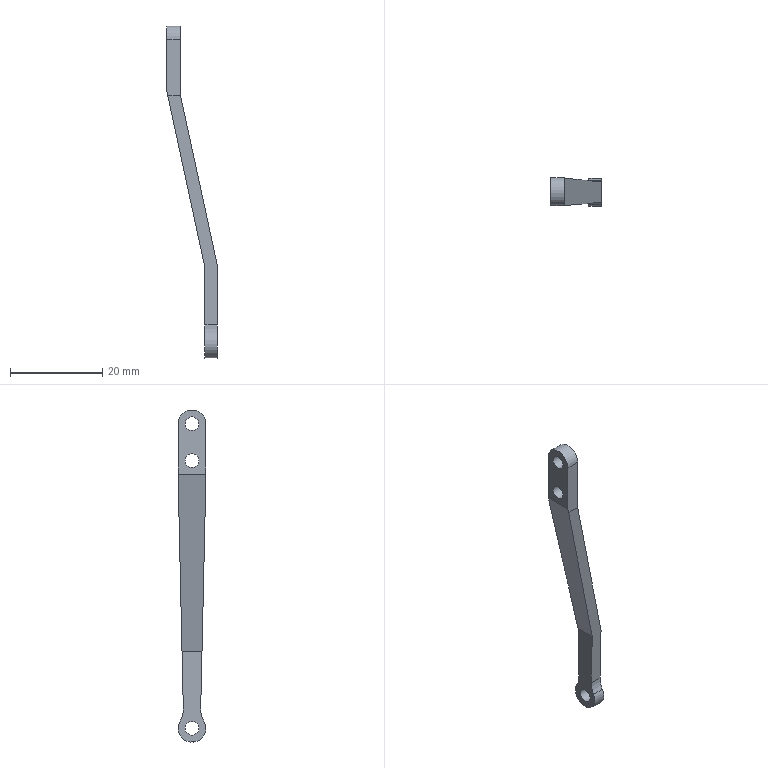Part | STEP file | 2-18 | 1 solid | 17 faces | box 11 x 6 x 72 mm | volume 957.208 mm3 | plane 10 | cylinder 7 | commonest cylinder face diameters 3 x3 6 x2 10 x2
STEP:
#1=CARTESIAN_POINT('',(0.,0.,0.));
#2=DIRECTION('',(0.,0.,1.));
#3=DIRECTION('',(1.,0.,0.));
#4=AXIS2_PLACEMENT_3D('',#1,#2,#3);
#5=CARTESIAN_POINT('',(-7.5,3.,0.));
#6=VERTEX_POINT('',#5);
#7=CARTESIAN_POINT('',(-7.5,-3.,0.));
#8=VERTEX_POINT('',#7);
#9=CARTESIAN_POINT('',(-7.5,0.,0.));
#10=DIRECTION('',(1.,0.,0.));
#11=DIRECTION('',(0.,1.,0.));
#12=AXIS2_PLACEMENT_3D('',#9,#10,#11);
#13=CIRCLE('',#12,3.);
#14=CARTESIAN_POINT('',(-7.5,32.591,-33.464));
#15=DIRECTION('',(1.,0.,0.));
#16=DIRECTION('',(0.,1.,0.));
#17=AXIS2_PLACEMENT_3D('',#14,#15,#16);
#18=PLANE('',#17);
#19=CARTESIAN_POINT('',(-32.591,33.464));
#20=DIRECTION('',(1.,0.));
#21=AXIS2_PLACEMENT_2D('',#19,#20);
#22=CIRCLE('',#21,3.);
#23=(GEOMETRIC_REPRESENTATION_CONTEXT(2)PARAMETRIC_REPRESENTATION_CONTEXT()REPRESENTATION_CONTEXT('',''));
#24=DEFINITIONAL_REPRESENTATION('',(#22),#23);
#25=PCURVE('',#18,#24);
#26=CARTESIAN_POINT('',(7.5,0.,0.));
#27=DIRECTION('',(-1.,0.,0.));
#28=DIRECTION('',(0.,1.,0.));
#29=AXIS2_PLACEMENT_3D('',#26,#27,#28);
#30=CYLINDRICAL_SURFACE('',#29,3.);
#31=CARTESIAN_POINT('',(6.283,15.));
#32=DIRECTION('',(-1.,0.));
#33=VECTOR('',#32,1.);
#34=LINE('',#31,#33);
#35=(GEOMETRIC_REPRESENTATION_CONTEXT(2)PARAMETRIC_REPRESENTATION_CONTEXT()REPRESENTATION_CONTEXT('',''));
#36=DEFINITIONAL_REPRESENTATION('',(#34),#35);
#37=PCURVE('',#30,#36);
#38=SURFACE_CURVE('',#13,(#25,#37),.PCURVE_S1.);
#39=EDGE_CURVE('',#6,#8,#38,.T.);
#40=ORIENTED_EDGE('',*,*,#39,.T.);
#41=CARTESIAN_POINT('',(-7.5,-3.,-10.901));
#42=VERTEX_POINT('',#41);
#43=CARTESIAN_POINT('',(-7.5,-3.,0.));
#44=DIRECTION('',(0.,0.,-1.));
#45=VECTOR('',#44,1.);
#46=LINE('',#43,#45);
#47=CARTESIAN_POINT('',(-35.591,33.464));
#48=DIRECTION('',(0.,-1.));
#49=VECTOR('',#48,1.);
#50=LINE('',#47,#49);
#51=(GEOMETRIC_REPRESENTATION_CONTEXT(2)PARAMETRIC_REPRESENTATION_CONTEXT()REPRESENTATION_CONTEXT('',''));
#52=DEFINITIONAL_REPRESENTATION('',(#50),#51);
#53=PCURVE('',#18,#52);
#54=CARTESIAN_POINT('',(0.,-3.,-6.));
#55=DIRECTION('',(0.,1.,0.));
#56=DIRECTION('',(0.,0.,-1.));
#57=AXIS2_PLACEMENT_3D('',#54,#55,#56);
#58=PLANE('',#57);
#59=CARTESIAN_POINT('',(-6.,7.5));
#60=DIRECTION('',(1.,0.));
#61=VECTOR('',#60,1.);
#62=LINE('',#59,#61);
#63=(GEOMETRIC_REPRESENTATION_CONTEXT(2)PARAMETRIC_REPRESENTATION_CONTEXT()REPRESENTATION_CONTEXT('',''));
#64=DEFINITIONAL_REPRESENTATION('',(#62),#63);
#65=PCURVE('',#58,#64);
#66=SURFACE_CURVE('',#46,(#53,#65),.PCURVE_S1.);
#67=EDGE_CURVE('',#8,#42,#66,.T.);
#68=ORIENTED_EDGE('',*,*,#67,.T.);
#69=CARTESIAN_POINT('',(-7.5,3.,-10.901));
#70=VERTEX_POINT('',#69);
#71=CARTESIAN_POINT('',(-7.5,3.,-10.901));
#72=DIRECTION('',(0.,-1.,0.));
#73=VECTOR('',#72,1.);
#74=LINE('',#71,#73);
#75=CARTESIAN_POINT('',(-29.591,22.563));
#76=DIRECTION('',(-1.,0.));
#77=VECTOR('',#76,1.);
#78=LINE('',#75,#77);
#79=(GEOMETRIC_REPRESENTATION_CONTEXT(2)PARAMETRIC_REPRESENTATION_CONTEXT()REPRESENTATION_CONTEXT('',''));
#80=DEFINITIONAL_REPRESENTATION('',(#78),#79);
#81=PCURVE('',#18,#80);
#82=CARTESIAN_POINT('',(-3.35,0.,-30.095));
#83=DIRECTION('',(-0.9774,0.,-0.2113));
#84=DIRECTION('',(0.2113,0.,-0.9774));
#85=AXIS2_PLACEMENT_3D('',#82,#83,#84);
#86=PLANE('',#85);
#87=CARTESIAN_POINT('',(-19.637,-3.));
#88=DIRECTION('',(0.,1.));
#89=VECTOR('',#88,1.);
#90=LINE('',#87,#89);
#91=(GEOMETRIC_REPRESENTATION_CONTEXT(2)PARAMETRIC_REPRESENTATION_CONTEXT()REPRESENTATION_CONTEXT('',''));
#92=DEFINITIONAL_REPRESENTATION('',(#90),#91);
#93=PCURVE('',#86,#92);
#94=SURFACE_CURVE('',#74,(#81,#93),.PCURVE_S1.);
#95=EDGE_CURVE('',#70,#42,#94,.T.);
#96=ORIENTED_EDGE('',*,*,#95,.F.);
#97=CARTESIAN_POINT('',(-7.5,3.,-10.901));
#98=DIRECTION('',(0.,0.,1.));
#99=VECTOR('',#98,1.);
#100=LINE('',#97,#99);
#101=CARTESIAN_POINT('',(-29.591,22.563));
#102=DIRECTION('',(0.,1.));
#103=VECTOR('',#102,1.);
#104=LINE('',#101,#103);
#105=(GEOMETRIC_REPRESENTATION_CONTEXT(2)PARAMETRIC_REPRESENTATION_CONTEXT()REPRESENTATION_CONTEXT('',''));
#106=DEFINITIONAL_REPRESENTATION('',(#104),#105);
#107=PCURVE('',#18,#106);
#108=CARTESIAN_POINT('',(0.,3.,-6.));
#109=DIRECTION('',(0.,-1.,0.));
#110=DIRECTION('',(0.,0.,1.));
#111=AXIS2_PLACEMENT_3D('',#108,#109,#110);
#112=PLANE('',#111);
#113=CARTESIAN_POINT('',(-4.901,7.5));
#114=DIRECTION('',(1.,0.));
#115=VECTOR('',#114,1.);
#116=LINE('',#113,#115);
#117=(GEOMETRIC_REPRESENTATION_CONTEXT(2)PARAMETRIC_REPRESENTATION_CONTEXT()REPRESENTATION_CONTEXT('',''));
#118=DEFINITIONAL_REPRESENTATION('',(#116),#117);
#119=PCURVE('',#112,#118);
#120=SURFACE_CURVE('',#100,(#107,#119),.PCURVE_S1.);
#121=EDGE_CURVE('',#70,#6,#120,.T.);
#122=ORIENTED_EDGE('',*,*,#121,.T.);
#123=EDGE_LOOP('',(#40,#68,#96,#122));
#124=FACE_BOUND('',#123,.F.);
#125=CARTESIAN_POINT('',(-7.5,1.5,0.));
#126=VERTEX_POINT('',#125);
#127=CARTESIAN_POINT('',(-7.5,0.,0.));
#128=DIRECTION('',(-1.,0.,0.));
#129=DIRECTION('',(0.,1.,0.));
#130=AXIS2_PLACEMENT_3D('',#127,#128,#129);
#131=CIRCLE('',#130,1.5);
#132=CARTESIAN_POINT('',(-31.091,33.464));
#133=CARTESIAN_POINT('',(-31.091,30.866));
#134=CARTESIAN_POINT('',(-33.341,32.165));
#135=CARTESIAN_POINT('',(-35.591,33.464));
#136=CARTESIAN_POINT('',(-33.341,34.763));
#137=CARTESIAN_POINT('',(-31.091,36.062));
#138=CARTESIAN_POINT('',(-31.091,33.464));
#139=(BOUNDED_CURVE()B_SPLINE_CURVE(2,(#132,#133,#134,#135,#136,#137,#138),.UNSPECIFIED.,.T.,.F.)B_SPLINE_CURVE_WITH_KNOTS((1,2,2,2,2,1),(-2.094,0.,2.094,4.189,6.283,8.378),.UNSPECIFIED.)CURVE()GEOMETRIC_REPRESENTATION_ITEM()RATIONAL_B_SPLINE_CURVE((1.,0.5,1.,0.5,1.,0.5,1.))REPRESENTATION_ITEM(''));
#140=(GEOMETRIC_REPRESENTATION_CONTEXT(2)PARAMETRIC_REPRESENTATION_CONTEXT()REPRESENTATION_CONTEXT('',''));
#141=DEFINITIONAL_REPRESENTATION('',(#139),#140);
#142=PCURVE('',#18,#141);
#143=CARTESIAN_POINT('',(7.5,0.,0.));
#144=DIRECTION('',(-1.,0.,0.));
#145=DIRECTION('',(0.,1.,0.));
#146=AXIS2_PLACEMENT_3D('',#143,#144,#145);
#147=CYLINDRICAL_SURFACE('',#146,1.5);
#148=CARTESIAN_POINT('',(0.,15.));
#149=DIRECTION('',(1.,0.));
#150=VECTOR('',#149,1.);
#151=LINE('',#148,#150);
#152=(GEOMETRIC_REPRESENTATION_CONTEXT(2)PARAMETRIC_REPRESENTATION_CONTEXT()REPRESENTATION_CONTEXT('',''));
#153=DEFINITIONAL_REPRESENTATION('',(#151),#152);
#154=PCURVE('',#147,#153);
#155=SURFACE_CURVE('',#131,(#142,#154),.PCURVE_S1.);
#156=EDGE_CURVE('',#126,#126,#155,.T.);
#157=ORIENTED_EDGE('',*,*,#156,.T.);
#158=EDGE_LOOP('',(#157));
#159=FACE_BOUND('',#158,.F.);
#160=CARTESIAN_POINT('',(-7.5,1.5,-8.));
#161=VERTEX_POINT('',#160);
#162=CARTESIAN_POINT('',(-7.5,0.,-8.));
#163=DIRECTION('',(-1.,0.,0.));
#164=DIRECTION('',(0.,1.,0.));
#165=AXIS2_PLACEMENT_3D('',#162,#163,#164);
#166=CIRCLE('',#165,1.5);
#167=CARTESIAN_POINT('',(-31.091,25.464));
#168=CARTESIAN_POINT('',(-31.091,22.866));
#169=CARTESIAN_POINT('',(-33.341,24.165));
#170=CARTESIAN_POINT('',(-35.591,25.464));
#171=CARTESIAN_POINT('',(-33.341,26.763));
#172=CARTESIAN_POINT('',(-31.091,28.062));
#173=CARTESIAN_POINT('',(-31.091,25.464));
#174=(BOUNDED_CURVE()B_SPLINE_CURVE(2,(#167,#168,#169,#170,#171,#172,#173),.UNSPECIFIED.,.T.,.F.)B_SPLINE_CURVE_WITH_KNOTS((1,2,2,2,2,1),(-2.094,0.,2.094,4.189,6.283,8.378),.UNSPECIFIED.)CURVE()GEOMETRIC_REPRESENTATION_ITEM()RATIONAL_B_SPLINE_CURVE((1.,0.5,1.,0.5,1.,0.5,1.))REPRESENTATION_ITEM(''));
#175=(GEOMETRIC_REPRESENTATION_CONTEXT(2)PARAMETRIC_REPRESENTATION_CONTEXT()REPRESENTATION_CONTEXT('',''));
#176=DEFINITIONAL_REPRESENTATION('',(#174),#175);
#177=PCURVE('',#18,#176);
#178=CARTESIAN_POINT('',(7.5,0.,-8.));
#179=DIRECTION('',(-1.,0.,0.));
#180=DIRECTION('',(0.,1.,0.));
#181=AXIS2_PLACEMENT_3D('',#178,#179,#180);
#182=CYLINDRICAL_SURFACE('',#181,1.5);
#183=CARTESIAN_POINT('',(0.,15.));
#184=DIRECTION('',(1.,0.));
#185=VECTOR('',#184,1.);
#186=LINE('',#183,#185);
#187=(GEOMETRIC_REPRESENTATION_CONTEXT(2)PARAMETRIC_REPRESENTATION_CONTEXT()REPRESENTATION_CONTEXT('',''));
#188=DEFINITIONAL_REPRESENTATION('',(#186),#187);
#189=PCURVE('',#182,#188);
#190=SURFACE_CURVE('',#166,(#177,#189),.PCURVE_S1.);
#191=EDGE_CURVE('',#161,#161,#190,.T.);
#192=ORIENTED_EDGE('',*,*,#191,.T.);
#193=EDGE_LOOP('',(#192));
#194=FACE_BOUND('',#193,.F.);
#195=ADVANCED_FACE('',(#124,#159,#194),#18,.F.);
#196=CARTESIAN_POINT('',(-4.5,-3.,0.));
#197=VERTEX_POINT('',#196);
#198=CARTESIAN_POINT('',(-4.5,-3.,0.));
#199=DIRECTION('',(-1.,0.,0.));
#200=VECTOR('',#199,1.);
#201=LINE('',#198,#200);
#202=CARTESIAN_POINT('',(3.142,12.));
#203=DIRECTION('',(0.,1.));
#204=VECTOR('',#203,1.);
#205=LINE('',#202,#204);
#206=(GEOMETRIC_REPRESENTATION_CONTEXT(2)PARAMETRIC_REPRESENTATION_CONTEXT()REPRESENTATION_CONTEXT('',''));
#207=DEFINITIONAL_REPRESENTATION('',(#205),#206);
#208=PCURVE('',#30,#207);
#209=CARTESIAN_POINT('',(-6.,4.5));
#210=DIRECTION('',(0.,1.));
#211=VECTOR('',#210,1.);
#212=LINE('',#209,#211);
#213=(GEOMETRIC_REPRESENTATION_CONTEXT(2)PARAMETRIC_REPRESENTATION_CONTEXT()REPRESENTATION_CONTEXT('',''));
#214=DEFINITIONAL_REPRESENTATION('',(#212),#213);
#215=PCURVE('',#58,#214);
#216=SURFACE_CURVE('',#201,(#208,#215),.PCURVE_S1.);
#217=EDGE_CURVE('',#197,#8,#216,.T.);
#218=ORIENTED_EDGE('',*,*,#217,.F.);
#219=CARTESIAN_POINT('',(-4.5,3.,0.));
#220=VERTEX_POINT('',#219);
#221=CARTESIAN_POINT('',(-4.5,0.,0.));
#222=DIRECTION('',(1.,0.,0.));
#223=DIRECTION('',(0.,1.,0.));
#224=AXIS2_PLACEMENT_3D('',#221,#222,#223);
#225=CIRCLE('',#224,3.);
#226=CARTESIAN_POINT('',(6.283,12.));
#227=DIRECTION('',(-1.,0.));
#228=VECTOR('',#227,1.);
#229=LINE('',#226,#228);
#230=(GEOMETRIC_REPRESENTATION_CONTEXT(2)PARAMETRIC_REPRESENTATION_CONTEXT()REPRESENTATION_CONTEXT('',''));
#231=DEFINITIONAL_REPRESENTATION('',(#229),#230);
#232=PCURVE('',#30,#231);
#233=CARTESIAN_POINT('',(-4.5,0.,-4.5));
#234=DIRECTION('',(1.,0.,0.));
#235=DIRECTION('',(0.,0.,1.));
#236=AXIS2_PLACEMENT_3D('',#233,#234,#235);
#237=PLANE('',#236);
#238=CARTESIAN_POINT('',(4.5,0.));
#239=DIRECTION('',(0.,-1.));
#240=AXIS2_PLACEMENT_2D('',#238,#239);
#241=CIRCLE('',#240,3.);
#242=(GEOMETRIC_REPRESENTATION_CONTEXT(2)PARAMETRIC_REPRESENTATION_CONTEXT()REPRESENTATION_CONTEXT('',''));
#243=DEFINITIONAL_REPRESENTATION('',(#241),#242);
#244=PCURVE('',#237,#243);
#245=SURFACE_CURVE('',#225,(#232,#244),.PCURVE_S1.);
#246=EDGE_CURVE('',#220,#197,#245,.T.);
#247=ORIENTED_EDGE('',*,*,#246,.F.);
#248=CARTESIAN_POINT('',(-4.5,3.,0.));
#249=DIRECTION('',(-1.,0.,0.));
#250=VECTOR('',#249,1.);
#251=LINE('',#248,#250);
#252=CARTESIAN_POINT('',(6.283,12.));
#253=DIRECTION('',(0.,1.));
#254=VECTOR('',#253,1.);
#255=LINE('',#252,#254);
#256=(GEOMETRIC_REPRESENTATION_CONTEXT(2)PARAMETRIC_REPRESENTATION_CONTEXT()REPRESENTATION_CONTEXT('',''));
#257=DEFINITIONAL_REPRESENTATION('',(#255),#256);
#258=PCURVE('',#30,#257);
#259=CARTESIAN_POINT('',(6.,4.5));
#260=DIRECTION('',(0.,1.));
#261=VECTOR('',#260,1.);
#262=LINE('',#259,#261);
#263=(GEOMETRIC_REPRESENTATION_CONTEXT(2)PARAMETRIC_REPRESENTATION_CONTEXT()REPRESENTATION_CONTEXT('',''));
#264=DEFINITIONAL_REPRESENTATION('',(#262),#263);
#265=PCURVE('',#112,#264);
#266=SURFACE_CURVE('',#251,(#258,#265),.PCURVE_S1.);
#267=EDGE_CURVE('',#220,#6,#266,.T.);
#268=ORIENTED_EDGE('',*,*,#267,.T.);
#269=ORIENTED_EDGE('',*,*,#39,.T.);
#270=EDGE_LOOP('',(#218,#247,#268,#269));
#271=FACE_BOUND('',#270,.T.);
#272=ADVANCED_FACE('',(#271),#30,.T.);
#273=ORIENTED_EDGE('',*,*,#217,.F.);
#274=CARTESIAN_POINT('',(-4.5,-3.,-12.));
#275=VERTEX_POINT('',#274);
#276=CARTESIAN_POINT('',(-4.5,-3.,0.));
#277=DIRECTION('',(0.,0.,-1.));
#278=VECTOR('',#277,1.);
#279=LINE('',#276,#278);
#280=CARTESIAN_POINT('',(-6.,4.5));
#281=DIRECTION('',(1.,0.));
#282=VECTOR('',#281,1.);
#283=LINE('',#280,#282);
#284=(GEOMETRIC_REPRESENTATION_CONTEXT(2)PARAMETRIC_REPRESENTATION_CONTEXT()REPRESENTATION_CONTEXT('',''));
#285=DEFINITIONAL_REPRESENTATION('',(#283),#284);
#286=PCURVE('',#58,#285);
#287=CARTESIAN_POINT('',(4.5,3.));
#288=DIRECTION('',(-1.,0.));
#289=VECTOR('',#288,1.);
#290=LINE('',#287,#289);
#291=(GEOMETRIC_REPRESENTATION_CONTEXT(2)PARAMETRIC_REPRESENTATION_CONTEXT()REPRESENTATION_CONTEXT('',''));
#292=DEFINITIONAL_REPRESENTATION('',(#290),#291);
#293=PCURVE('',#237,#292);
#294=SURFACE_CURVE('',#279,(#286,#293),.PCURVE_S1.);
#295=EDGE_CURVE('',#197,#275,#294,.T.);
#296=ORIENTED_EDGE('',*,*,#295,.T.);
#297=CARTESIAN_POINT('',(-7.262,-3.,-12.));
#298=VERTEX_POINT('',#297);
#299=CARTESIAN_POINT('',(-4.5,-3.,-12.));
#300=DIRECTION('',(-1.,0.,0.));
#301=VECTOR('',#300,1.);
#302=LINE('',#299,#301);
#303=CARTESIAN_POINT('',(6.,4.5));
#304=DIRECTION('',(0.,1.));
#305=VECTOR('',#304,1.);
#306=LINE('',#303,#305);
#307=(GEOMETRIC_REPRESENTATION_CONTEXT(2)PARAMETRIC_REPRESENTATION_CONTEXT()REPRESENTATION_CONTEXT('',''));
#308=DEFINITIONAL_REPRESENTATION('',(#306),#307);
#309=PCURVE('',#58,#308);
#310=CARTESIAN_POINT('',(0.,-2.443,-36.907));
#311=DIRECTION('',(0.,0.9997,0.02236));
#312=DIRECTION('',(0.,0.02236,-0.9997));
#313=AXIS2_PLACEMENT_3D('',#310,#311,#312);
#314=PLANE('',#313);
#315=CARTESIAN_POINT('',(-24.913,4.5));
#316=DIRECTION('',(0.,1.));
#317=VECTOR('',#316,1.);
#318=LINE('',#315,#317);
#319=(GEOMETRIC_REPRESENTATION_CONTEXT(2)PARAMETRIC_REPRESENTATION_CONTEXT()REPRESENTATION_CONTEXT('',''));
#320=DEFINITIONAL_REPRESENTATION('',(#318),#319);
#321=PCURVE('',#314,#320);
#322=SURFACE_CURVE('',#302,(#309,#321),.PCURVE_S1.);
#323=EDGE_CURVE('',#275,#298,#322,.T.);
#324=ORIENTED_EDGE('',*,*,#323,.T.);
#325=CARTESIAN_POINT('',(-7.262,-3.,-12.));
#326=DIRECTION('',(-0.2113,0.,0.9774));
#327=VECTOR('',#326,1.);
#328=LINE('',#325,#327);
#329=CARTESIAN_POINT('',(6.,7.262));
#330=DIRECTION('',(-0.9774,0.2113));
#331=VECTOR('',#330,1.);
#332=LINE('',#329,#331);
#333=(GEOMETRIC_REPRESENTATION_CONTEXT(2)PARAMETRIC_REPRESENTATION_CONTEXT()REPRESENTATION_CONTEXT('',''));
#334=DEFINITIONAL_REPRESENTATION('',(#332),#333);
#335=PCURVE('',#58,#334);
#336=CARTESIAN_POINT('',(-18.513,3.));
#337=DIRECTION('',(-1.,0.));
#338=VECTOR('',#337,1.);
#339=LINE('',#336,#338);
#340=(GEOMETRIC_REPRESENTATION_CONTEXT(2)PARAMETRIC_REPRESENTATION_CONTEXT()REPRESENTATION_CONTEXT('',''));
#341=DEFINITIONAL_REPRESENTATION('',(#339),#340);
#342=PCURVE('',#86,#341);
#343=SURFACE_CURVE('',#328,(#335,#342),.PCURVE_S1.);
#344=EDGE_CURVE('',#298,#42,#343,.T.);
#345=ORIENTED_EDGE('',*,*,#344,.T.);
#346=ORIENTED_EDGE('',*,*,#67,.F.);
#347=EDGE_LOOP('',(#273,#296,#324,#345,#346));
#348=FACE_BOUND('',#347,.F.);
#349=ADVANCED_FACE('',(#348),#58,.F.);
#350=ORIENTED_EDGE('',*,*,#323,.F.);
#351=CARTESIAN_POINT('',(3.5,-2.172,-49.));
#352=VERTEX_POINT('',#351);
#353=CARTESIAN_POINT('',(-4.5,-3.,-12.));
#354=DIRECTION('',(0.2113,0.02186,-0.9772));
#355=VECTOR('',#354,1.);
#356=LINE('',#353,#355);
#357=CARTESIAN_POINT('',(-24.913,4.5));
#358=DIRECTION('',(0.9774,-0.2113));
#359=VECTOR('',#358,1.);
#360=LINE('',#357,#359);
#361=(GEOMETRIC_REPRESENTATION_CONTEXT(2)PARAMETRIC_REPRESENTATION_CONTEXT()REPRESENTATION_CONTEXT('',''));
#362=DEFINITIONAL_REPRESENTATION('',(#360),#361);
#363=PCURVE('',#314,#362);
#364=CARTESIAN_POINT('',(-0.5,0.,-30.5));
#365=DIRECTION('',(0.9774,0.,0.2113));
#366=DIRECTION('',(-0.2113,0.,0.9774));
#367=AXIS2_PLACEMENT_3D('',#364,#365,#366);
#368=PLANE('',#367);
#369=CARTESIAN_POINT('',(18.927,3.));
#370=DIRECTION('',(-0.9998,-0.02186));
#371=VECTOR('',#370,1.);
#372=LINE('',#369,#371);
#373=(GEOMETRIC_REPRESENTATION_CONTEXT(2)PARAMETRIC_REPRESENTATION_CONTEXT()REPRESENTATION_CONTEXT('',''));
#374=DEFINITIONAL_REPRESENTATION('',(#372),#373);
#375=PCURVE('',#368,#374);
#376=SURFACE_CURVE('',#356,(#363,#375),.PCURVE_S1.);
#377=EDGE_CURVE('',#275,#352,#376,.T.);
#378=ORIENTED_EDGE('',*,*,#377,.T.);
#379=CARTESIAN_POINT('',(3.5,-1.886,-61.814));
#380=VERTEX_POINT('',#379);
#381=CARTESIAN_POINT('',(3.5,-2.172,-49.));
#382=DIRECTION('',(0.,0.02236,-0.9997));
#383=VECTOR('',#382,1.);
#384=LINE('',#381,#383);
#385=CARTESIAN_POINT('',(12.096,-3.5));
#386=DIRECTION('',(1.,0.));
#387=VECTOR('',#386,1.);
#388=LINE('',#385,#387);
#389=(GEOMETRIC_REPRESENTATION_CONTEXT(2)PARAMETRIC_REPRESENTATION_CONTEXT()REPRESENTATION_CONTEXT('',''));
#390=DEFINITIONAL_REPRESENTATION('',(#388),#389);
#391=PCURVE('',#314,#390);
#392=CARTESIAN_POINT('',(3.5,0.,-59.));
#393=DIRECTION('',(1.,0.,0.));
#394=DIRECTION('',(0.,0.,1.));
#395=AXIS2_PLACEMENT_3D('',#392,#393,#394);
#396=PLANE('',#395);
#397=CARTESIAN_POINT('',(10.,2.172));
#398=DIRECTION('',(-0.9997,-0.02236));
#399=VECTOR('',#398,1.);
#400=LINE('',#397,#399);
#401=(GEOMETRIC_REPRESENTATION_CONTEXT(2)PARAMETRIC_REPRESENTATION_CONTEXT()REPRESENTATION_CONTEXT('',''));
#402=DEFINITIONAL_REPRESENTATION('',(#400),#401);
#403=PCURVE('',#396,#402);
#404=SURFACE_CURVE('',#384,(#391,#403),.PCURVE_S1.);
#405=EDGE_CURVE('',#352,#380,#404,.T.);
#406=ORIENTED_EDGE('',*,*,#405,.T.);
#407=CARTESIAN_POINT('',(0.8,-1.886,-61.814));
#408=VERTEX_POINT('',#407);
#409=CARTESIAN_POINT('',(3.5,-1.886,-61.814));
#410=DIRECTION('',(-1.,0.,0.));
#411=VECTOR('',#410,1.);
#412=LINE('',#409,#411);
#413=CARTESIAN_POINT('',(24.913,-3.5));
#414=DIRECTION('',(0.,1.));
#415=VECTOR('',#414,1.);
#416=LINE('',#413,#415);
#417=(GEOMETRIC_REPRESENTATION_CONTEXT(2)PARAMETRIC_REPRESENTATION_CONTEXT()REPRESENTATION_CONTEXT('',''));
#418=DEFINITIONAL_REPRESENTATION('',(#416),#417);
#419=PCURVE('',#314,#418);
#420=CARTESIAN_POINT('',(7.5,-6.885,-61.925));
#421=DIRECTION('',(-1.,0.,0.));
#422=DIRECTION('',(0.,0.9997,0.02236));
#423=AXIS2_PLACEMENT_3D('',#420,#421,#422);
#424=CYLINDRICAL_SURFACE('',#423,5.);
#425=CARTESIAN_POINT('',(0.,4.));
#426=DIRECTION('',(0.,1.));
#427=VECTOR('',#426,1.);
#428=LINE('',#425,#427);
#429=(GEOMETRIC_REPRESENTATION_CONTEXT(2)PARAMETRIC_REPRESENTATION_CONTEXT()REPRESENTATION_CONTEXT('',''));
#430=DEFINITIONAL_REPRESENTATION('',(#428),#429);
#431=PCURVE('',#424,#430);
#432=SURFACE_CURVE('',#412,(#419,#431),.PCURVE_S1.);
#433=EDGE_CURVE('',#380,#408,#432,.T.);
#434=ORIENTED_EDGE('',*,*,#433,.T.);
#435=CARTESIAN_POINT('',(0.8,-2.166,-49.289));
#436=VERTEX_POINT('',#435);
#437=CARTESIAN_POINT('',(0.8,-1.886,-61.814));
#438=DIRECTION('',(0.,-0.02236,0.9997));
#439=VECTOR('',#438,1.);
#440=LINE('',#437,#439);
#441=CARTESIAN_POINT('',(24.913,-0.8));
#442=DIRECTION('',(-1.,0.));
#443=VECTOR('',#442,1.);
#444=LINE('',#441,#443);
#445=(GEOMETRIC_REPRESENTATION_CONTEXT(2)PARAMETRIC_REPRESENTATION_CONTEXT()REPRESENTATION_CONTEXT('',''));
#446=DEFINITIONAL_REPRESENTATION('',(#444),#445);
#447=PCURVE('',#314,#446);
#448=CARTESIAN_POINT('',(0.8,0.,-59.144));
#449=DIRECTION('',(-1.,0.,0.));
#450=DIRECTION('',(0.,0.,-1.));
#451=AXIS2_PLACEMENT_3D('',#448,#449,#450);
#452=PLANE('',#451);
#453=CARTESIAN_POINT('',(2.669,1.886));
#454=DIRECTION('',(-0.9997,0.02236));
#455=VECTOR('',#454,1.);
#456=LINE('',#453,#455);
#457=(GEOMETRIC_REPRESENTATION_CONTEXT(2)PARAMETRIC_REPRESENTATION_CONTEXT()REPRESENTATION_CONTEXT('',''));
#458=DEFINITIONAL_REPRESENTATION('',(#456),#457);
#459=PCURVE('',#452,#458);
#460=SURFACE_CURVE('',#440,(#447,#459),.PCURVE_S1.);
#461=EDGE_CURVE('',#408,#436,#460,.T.);
#462=ORIENTED_EDGE('',*,*,#461,.T.);
#463=CARTESIAN_POINT('',(0.8,-2.166,-49.289));
#464=DIRECTION('',(-0.2113,-0.02186,0.9772));
#465=VECTOR('',#464,1.);
#466=LINE('',#463,#465);
#467=CARTESIAN_POINT('',(12.385,-0.8));
#468=DIRECTION('',(-0.9774,0.2113));
#469=VECTOR('',#468,1.);
#470=LINE('',#467,#469);
#471=(GEOMETRIC_REPRESENTATION_CONTEXT(2)PARAMETRIC_REPRESENTATION_CONTEXT()REPRESENTATION_CONTEXT('',''));
#472=DEFINITIONAL_REPRESENTATION('',(#470),#471);
#473=PCURVE('',#314,#472);
#474=CARTESIAN_POINT('',(19.637,2.166));
#475=DIRECTION('',(-0.9998,0.02186));
#476=VECTOR('',#475,1.);
#477=LINE('',#474,#476);
#478=(GEOMETRIC_REPRESENTATION_CONTEXT(2)PARAMETRIC_REPRESENTATION_CONTEXT()REPRESENTATION_CONTEXT('',''));
#479=DEFINITIONAL_REPRESENTATION('',(#477),#478);
#480=PCURVE('',#86,#479);
#481=SURFACE_CURVE('',#466,(#473,#480),.PCURVE_S1.);
#482=EDGE_CURVE('',#436,#298,#481,.T.);
#483=ORIENTED_EDGE('',*,*,#482,.T.);
#484=EDGE_LOOP('',(#350,#378,#406,#434,#462,#483));
#485=FACE_BOUND('',#484,.F.);
#486=ADVANCED_FACE('',(#485),#314,.F.);
#487=ORIENTED_EDGE('',*,*,#433,.F.);
#488=CARTESIAN_POINT('',(3.5,-2.582,-64.472));
#489=VERTEX_POINT('',#488);
#490=CARTESIAN_POINT('',(3.5,-6.885,-61.925));
#491=DIRECTION('',(-1.,0.,0.));
#492=DIRECTION('',(0.,0.9997,0.02236));
#493=AXIS2_PLACEMENT_3D('',#490,#491,#492);
#494=CIRCLE('',#493,5.);
#495=CARTESIAN_POINT('',(0.,4.));
#496=DIRECTION('',(1.,0.));
#497=VECTOR('',#496,1.);
#498=LINE('',#495,#497);
#499=(GEOMETRIC_REPRESENTATION_CONTEXT(2)PARAMETRIC_REPRESENTATION_CONTEXT()REPRESENTATION_CONTEXT('',''));
#500=DEFINITIONAL_REPRESENTATION('',(#498),#499);
#501=PCURVE('',#424,#500);
#502=CARTESIAN_POINT('',(-2.814,1.886));
#503=CARTESIAN_POINT('',(-11.472,1.692));
#504=CARTESIAN_POINT('',(-7.31,9.287));
#505=CARTESIAN_POINT('',(-3.149,16.882));
#506=CARTESIAN_POINT('',(1.348,9.481));
#507=CARTESIAN_POINT('',(5.844,2.08));
#508=CARTESIAN_POINT('',(-2.814,1.886));
#509=(BOUNDED_CURVE()B_SPLINE_CURVE(2,(#502,#503,#504,#505,#506,#507,#508),.UNSPECIFIED.,.T.,.F.)B_SPLINE_CURVE_WITH_KNOTS((1,2,2,2,2,1),(-2.094,0.,2.094,4.189,6.283,8.378),.UNSPECIFIED.)CURVE()GEOMETRIC_REPRESENTATION_ITEM()RATIONAL_B_SPLINE_CURVE((1.,0.5,1.,0.5,1.,0.5,1.))REPRESENTATION_ITEM(''));
#510=(GEOMETRIC_REPRESENTATION_CONTEXT(2)PARAMETRIC_REPRESENTATION_CONTEXT()REPRESENTATION_CONTEXT('',''));
#511=DEFINITIONAL_REPRESENTATION('',(#509),#510);
#512=PCURVE('',#396,#511);
#513=SURFACE_CURVE('',#494,(#501,#512),.PCURVE_S1.);
#514=EDGE_CURVE('',#380,#489,#513,.T.);
#515=ORIENTED_EDGE('',*,*,#514,.T.);
#516=CARTESIAN_POINT('',(0.8,-2.582,-64.472));
#517=VERTEX_POINT('',#516);
#518=CARTESIAN_POINT('',(3.5,-2.582,-64.472));
#519=DIRECTION('',(-1.,0.,0.));
#520=VECTOR('',#519,1.);
#521=LINE('',#518,#520);
#522=CARTESIAN_POINT('',(0.5568,4.));
#523=DIRECTION('',(0.,1.));
#524=VECTOR('',#523,1.);
#525=LINE('',#522,#524);
#526=(GEOMETRIC_REPRESENTATION_CONTEXT(2)PARAMETRIC_REPRESENTATION_CONTEXT()REPRESENTATION_CONTEXT('',''));
#527=DEFINITIONAL_REPRESENTATION('',(#525),#526);
#528=PCURVE('',#424,#527);
#529=CARTESIAN_POINT('',(7.5,0.,-66.));
#530=DIRECTION('',(-1.,0.,0.));
#531=DIRECTION('',(0.,-0.8606,0.5093));
#532=AXIS2_PLACEMENT_3D('',#529,#530,#531);
#533=CYLINDRICAL_SURFACE('',#532,3.);
#534=CARTESIAN_POINT('',(6.283,4.));
#535=DIRECTION('',(0.,1.));
#536=VECTOR('',#535,1.);
#537=LINE('',#534,#536);
#538=(GEOMETRIC_REPRESENTATION_CONTEXT(2)PARAMETRIC_REPRESENTATION_CONTEXT()REPRESENTATION_CONTEXT('',''));
#539=DEFINITIONAL_REPRESENTATION('',(#537),#538);
#540=PCURVE('',#533,#539);
#541=SURFACE_CURVE('',#521,(#528,#540),.PCURVE_S1.);
#542=EDGE_CURVE('',#489,#517,#541,.T.);
#543=ORIENTED_EDGE('',*,*,#542,.T.);
#544=CARTESIAN_POINT('',(0.8,-6.885,-61.925));
#545=DIRECTION('',(1.,0.,0.));
#546=DIRECTION('',(0.,0.8606,-0.5093));
#547=AXIS2_PLACEMENT_3D('',#544,#545,#546);
#548=CIRCLE('',#547,5.);
#549=CARTESIAN_POINT('',(0.5568,6.7));
#550=DIRECTION('',(-1.,0.));
#551=VECTOR('',#550,1.);
#552=LINE('',#549,#551);
#553=(GEOMETRIC_REPRESENTATION_CONTEXT(2)PARAMETRIC_REPRESENTATION_CONTEXT()REPRESENTATION_CONTEXT('',''));
#554=DEFINITIONAL_REPRESENTATION('',(#552),#553);
#555=PCURVE('',#424,#554);
#556=CARTESIAN_POINT('',(5.328,2.582));
#557=CARTESIAN_POINT('',(-2.125,-1.829));
#558=CARTESIAN_POINT('',(-2.219,6.831));
#559=CARTESIAN_POINT('',(-2.312,15.49));
#560=CARTESIAN_POINT('',(5.234,11.241));
#561=CARTESIAN_POINT('',(12.781,6.993));
#562=CARTESIAN_POINT('',(5.328,2.582));
#563=(BOUNDED_CURVE()B_SPLINE_CURVE(2,(#556,#557,#558,#559,#560,#561,#562),.UNSPECIFIED.,.T.,.F.)B_SPLINE_CURVE_WITH_KNOTS((1,2,2,2,2,1),(-2.094,0.,2.094,4.189,6.283,8.378),.UNSPECIFIED.)CURVE()GEOMETRIC_REPRESENTATION_ITEM()RATIONAL_B_SPLINE_CURVE((1.,0.5,1.,0.5,1.,0.5,1.))REPRESENTATION_ITEM(''));
#564=(GEOMETRIC_REPRESENTATION_CONTEXT(2)PARAMETRIC_REPRESENTATION_CONTEXT()REPRESENTATION_CONTEXT('',''));
#565=DEFINITIONAL_REPRESENTATION('',(#563),#564);
#566=PCURVE('',#452,#565);
#567=SURFACE_CURVE('',#548,(#555,#566),.PCURVE_S1.);
#568=EDGE_CURVE('',#517,#408,#567,.T.);
#569=ORIENTED_EDGE('',*,*,#568,.T.);
#570=EDGE_LOOP('',(#487,#515,#543,#569));
#571=FACE_BOUND('',#570,.F.);
#572=ADVANCED_FACE('',(#571),#424,.F.);
#573=CARTESIAN_POINT('',(0.8,2.582,-64.472));
#574=VERTEX_POINT('',#573);
#575=CARTESIAN_POINT('',(0.8,0.,-66.));
#576=DIRECTION('',(-1.,0.,0.));
#577=DIRECTION('',(0.,0.8606,0.5093));
#578=AXIS2_PLACEMENT_3D('',#575,#576,#577);
#579=CIRCLE('',#578,3.);
#580=CARTESIAN_POINT('',(2.073,6.7));
#581=DIRECTION('',(1.,0.));
#582=VECTOR('',#581,1.);
#583=LINE('',#580,#582);
#584=(GEOMETRIC_REPRESENTATION_CONTEXT(2)PARAMETRIC_REPRESENTATION_CONTEXT()REPRESENTATION_CONTEXT('',''));
#585=DEFINITIONAL_REPRESENTATION('',(#583),#584);
#586=PCURVE('',#533,#585);
#587=CARTESIAN_POINT('',(6.856,0.));
#588=DIRECTION('',(-0.5093,-0.8606));
#589=AXIS2_PLACEMENT_2D('',#587,#588);
#590=CIRCLE('',#589,3.);
#591=(GEOMETRIC_REPRESENTATION_CONTEXT(2)PARAMETRIC_REPRESENTATION_CONTEXT()REPRESENTATION_CONTEXT('',''));
#592=DEFINITIONAL_REPRESENTATION('',(#590),#591);
#593=PCURVE('',#452,#592);
#594=SURFACE_CURVE('',#579,(#586,#593),.PCURVE_S1.);
#595=EDGE_CURVE('',#574,#517,#594,.T.);
#596=ORIENTED_EDGE('',*,*,#595,.F.);
#597=CARTESIAN_POINT('',(3.5,2.582,-64.472));
#598=VERTEX_POINT('',#597);
#599=CARTESIAN_POINT('',(3.5,2.582,-64.472));
#600=DIRECTION('',(-1.,0.,0.));
#601=VECTOR('',#600,1.);
#602=LINE('',#599,#601);
#603=CARTESIAN_POINT('',(2.073,4.));
#604=DIRECTION('',(0.,1.));
#605=VECTOR('',#604,1.);
#606=LINE('',#603,#605);
#607=(GEOMETRIC_REPRESENTATION_CONTEXT(2)PARAMETRIC_REPRESENTATION_CONTEXT()REPRESENTATION_CONTEXT('',''));
#608=DEFINITIONAL_REPRESENTATION('',(#606),#607);
#609=PCURVE('',#533,#608);
#610=CARTESIAN_POINT('',(7.5,6.885,-61.925));
#611=DIRECTION('',(-1.,0.,0.));
#612=DIRECTION('',(0.,-0.8606,-0.5093));
#613=AXIS2_PLACEMENT_3D('',#610,#611,#612);
#614=CYLINDRICAL_SURFACE('',#613,5.);
#615=CARTESIAN_POINT('',(0.,4.));
#616=DIRECTION('',(0.,1.));
#617=VECTOR('',#616,1.);
#618=LINE('',#615,#617);
#619=(GEOMETRIC_REPRESENTATION_CONTEXT(2)PARAMETRIC_REPRESENTATION_CONTEXT()REPRESENTATION_CONTEXT('',''));
#620=DEFINITIONAL_REPRESENTATION('',(#618),#619);
#621=PCURVE('',#614,#620);
#622=SURFACE_CURVE('',#602,(#609,#621),.PCURVE_S1.);
#623=EDGE_CURVE('',#598,#574,#622,.T.);
#624=ORIENTED_EDGE('',*,*,#623,.F.);
#625=CARTESIAN_POINT('',(3.5,0.,-66.));
#626=DIRECTION('',(1.,0.,0.));
#627=DIRECTION('',(0.,-0.8606,0.5093));
#628=AXIS2_PLACEMENT_3D('',#625,#626,#627);
#629=CIRCLE('',#628,3.);
#630=CARTESIAN_POINT('',(6.283,4.));
#631=DIRECTION('',(-1.,0.));
#632=VECTOR('',#631,1.);
#633=LINE('',#630,#632);
#634=(GEOMETRIC_REPRESENTATION_CONTEXT(2)PARAMETRIC_REPRESENTATION_CONTEXT()REPRESENTATION_CONTEXT('',''));
#635=DEFINITIONAL_REPRESENTATION('',(#633),#634);
#636=PCURVE('',#533,#635);
#637=CARTESIAN_POINT('',(-7.,0.));
#638=DIRECTION('',(0.5093,0.8606));
#639=AXIS2_PLACEMENT_2D('',#637,#638);
#640=CIRCLE('',#639,3.);
#641=(GEOMETRIC_REPRESENTATION_CONTEXT(2)PARAMETRIC_REPRESENTATION_CONTEXT()REPRESENTATION_CONTEXT('',''));
#642=DEFINITIONAL_REPRESENTATION('',(#640),#641);
#643=PCURVE('',#396,#642);
#644=SURFACE_CURVE('',#629,(#636,#643),.PCURVE_S1.);
#645=EDGE_CURVE('',#489,#598,#644,.T.);
#646=ORIENTED_EDGE('',*,*,#645,.F.);
#647=ORIENTED_EDGE('',*,*,#542,.T.);
#648=EDGE_LOOP('',(#596,#624,#646,#647));
#649=FACE_BOUND('',#648,.T.);
#650=ADVANCED_FACE('',(#649),#533,.T.);
#651=ORIENTED_EDGE('',*,*,#623,.F.);
#652=CARTESIAN_POINT('',(3.5,1.886,-61.814));
#653=VERTEX_POINT('',#652);
#654=CARTESIAN_POINT('',(3.5,6.885,-61.925));
#655=DIRECTION('',(-1.,0.,0.));
#656=DIRECTION('',(0.,-0.8606,-0.5093));
#657=AXIS2_PLACEMENT_3D('',#654,#655,#656);
#658=CIRCLE('',#657,5.);
#659=CARTESIAN_POINT('',(0.,4.));
#660=DIRECTION('',(1.,0.));
#661=VECTOR('',#660,1.);
#662=LINE('',#659,#661);
#663=(GEOMETRIC_REPRESENTATION_CONTEXT(2)PARAMETRIC_REPRESENTATION_CONTEXT()REPRESENTATION_CONTEXT('',''));
#664=DEFINITIONAL_REPRESENTATION('',(#662),#663);
#665=PCURVE('',#614,#664);
#666=CARTESIAN_POINT('',(-5.472,-2.582));
#667=CARTESIAN_POINT('',(1.981,1.829));
#668=CARTESIAN_POINT('',(2.074,-6.831));
#669=CARTESIAN_POINT('',(2.168,-15.49));
#670=CARTESIAN_POINT('',(-5.379,-11.241));
#671=CARTESIAN_POINT('',(-12.925,-6.993));
#672=CARTESIAN_POINT('',(-5.472,-2.582));
#673=(BOUNDED_CURVE()B_SPLINE_CURVE(2,(#666,#667,#668,#669,#670,#671,#672),.UNSPECIFIED.,.T.,.F.)B_SPLINE_CURVE_WITH_KNOTS((1,2,2,2,2,1),(-2.094,0.,2.094,4.189,6.283,8.378),.UNSPECIFIED.)CURVE()GEOMETRIC_REPRESENTATION_ITEM()RATIONAL_B_SPLINE_CURVE((1.,0.5,1.,0.5,1.,0.5,1.))REPRESENTATION_ITEM(''));
#674=(GEOMETRIC_REPRESENTATION_CONTEXT(2)PARAMETRIC_REPRESENTATION_CONTEXT()REPRESENTATION_CONTEXT('',''));
#675=DEFINITIONAL_REPRESENTATION('',(#673),#674);
#676=PCURVE('',#396,#675);
#677=SURFACE_CURVE('',#658,(#665,#676),.PCURVE_S1.);
#678=EDGE_CURVE('',#598,#653,#677,.T.);
#679=ORIENTED_EDGE('',*,*,#678,.T.);
#680=CARTESIAN_POINT('',(0.8,1.886,-61.814));
#681=VERTEX_POINT('',#680);
#682=CARTESIAN_POINT('',(3.5,1.886,-61.814));
#683=DIRECTION('',(-1.,0.,0.));
#684=VECTOR('',#683,1.);
#685=LINE('',#682,#684);
#686=CARTESIAN_POINT('',(0.5568,4.));
#687=DIRECTION('',(0.,1.));
#688=VECTOR('',#687,1.);
#689=LINE('',#686,#688);
#690=(GEOMETRIC_REPRESENTATION_CONTEXT(2)PARAMETRIC_REPRESENTATION_CONTEXT()REPRESENTATION_CONTEXT('',''));
#691=DEFINITIONAL_REPRESENTATION('',(#689),#690);
#692=PCURVE('',#614,#691);
#693=CARTESIAN_POINT('',(0.,2.443,-36.907));
#694=DIRECTION('',(0.,-0.9997,0.02236));
#695=DIRECTION('',(0.,0.02236,0.9997));
#696=AXIS2_PLACEMENT_3D('',#693,#694,#695);
#697=PLANE('',#696);
#698=CARTESIAN_POINT('',(-24.913,-3.5));
#699=DIRECTION('',(0.,1.));
#700=VECTOR('',#699,1.);
#701=LINE('',#698,#700);
#702=(GEOMETRIC_REPRESENTATION_CONTEXT(2)PARAMETRIC_REPRESENTATION_CONTEXT()REPRESENTATION_CONTEXT('',''));
#703=DEFINITIONAL_REPRESENTATION('',(#701),#702);
#704=PCURVE('',#697,#703);
#705=SURFACE_CURVE('',#685,(#692,#704),.PCURVE_S1.);
#706=EDGE_CURVE('',#653,#681,#705,.T.);
#707=ORIENTED_EDGE('',*,*,#706,.T.);
#708=CARTESIAN_POINT('',(0.8,6.885,-61.925));
#709=DIRECTION('',(1.,0.,0.));
#710=DIRECTION('',(0.,-0.9997,0.02236));
#711=AXIS2_PLACEMENT_3D('',#708,#709,#710);
#712=CIRCLE('',#711,5.);
#713=CARTESIAN_POINT('',(0.5568,6.7));
#714=DIRECTION('',(-1.,0.));
#715=VECTOR('',#714,1.);
#716=LINE('',#713,#715);
#717=(GEOMETRIC_REPRESENTATION_CONTEXT(2)PARAMETRIC_REPRESENTATION_CONTEXT()REPRESENTATION_CONTEXT('',''));
#718=DEFINITIONAL_REPRESENTATION('',(#716),#717);
#719=PCURVE('',#614,#718);
#720=CARTESIAN_POINT('',(2.669,-1.886));
#721=CARTESIAN_POINT('',(11.327,-1.692));
#722=CARTESIAN_POINT('',(7.166,-9.287));
#723=CARTESIAN_POINT('',(3.005,-16.882));
#724=CARTESIAN_POINT('',(-1.492,-9.481));
#725=CARTESIAN_POINT('',(-5.989,-2.08));
#726=CARTESIAN_POINT('',(2.669,-1.886));
#727=(BOUNDED_CURVE()B_SPLINE_CURVE(2,(#720,#721,#722,#723,#724,#725,#726),.UNSPECIFIED.,.T.,.F.)B_SPLINE_CURVE_WITH_KNOTS((1,2,2,2,2,1),(-2.094,0.,2.094,4.189,6.283,8.378),.UNSPECIFIED.)CURVE()GEOMETRIC_REPRESENTATION_ITEM()RATIONAL_B_SPLINE_CURVE((1.,0.5,1.,0.5,1.,0.5,1.))REPRESENTATION_ITEM(''));
#728=(GEOMETRIC_REPRESENTATION_CONTEXT(2)PARAMETRIC_REPRESENTATION_CONTEXT()REPRESENTATION_CONTEXT('',''));
#729=DEFINITIONAL_REPRESENTATION('',(#727),#728);
#730=PCURVE('',#452,#729);
#731=SURFACE_CURVE('',#712,(#719,#730),.PCURVE_S1.);
#732=EDGE_CURVE('',#681,#574,#731,.T.);
#733=ORIENTED_EDGE('',*,*,#732,.T.);
#734=EDGE_LOOP('',(#651,#679,#707,#733));
#735=FACE_BOUND('',#734,.F.);
#736=ADVANCED_FACE('',(#735),#614,.F.);
#737=ORIENTED_EDGE('',*,*,#706,.F.);
#738=CARTESIAN_POINT('',(3.5,2.172,-49.));
#739=VERTEX_POINT('',#738);
#740=CARTESIAN_POINT('',(3.5,1.886,-61.814));
#741=DIRECTION('',(0.,0.02236,0.9997));
#742=VECTOR('',#741,1.);
#743=LINE('',#740,#742);
#744=CARTESIAN_POINT('',(-24.913,-3.5));
#745=DIRECTION('',(1.,0.));
#746=VECTOR('',#745,1.);
#747=LINE('',#744,#746);
#748=(GEOMETRIC_REPRESENTATION_CONTEXT(2)PARAMETRIC_REPRESENTATION_CONTEXT()REPRESENTATION_CONTEXT('',''));
#749=DEFINITIONAL_REPRESENTATION('',(#747),#748);
#750=PCURVE('',#697,#749);
#751=CARTESIAN_POINT('',(-2.814,-1.886));
#752=DIRECTION('',(0.9997,-0.02236));
#753=VECTOR('',#752,1.);
#754=LINE('',#751,#753);
#755=(GEOMETRIC_REPRESENTATION_CONTEXT(2)PARAMETRIC_REPRESENTATION_CONTEXT()REPRESENTATION_CONTEXT('',''));
#756=DEFINITIONAL_REPRESENTATION('',(#754),#755);
#757=PCURVE('',#396,#756);
#758=SURFACE_CURVE('',#743,(#750,#757),.PCURVE_S1.);
#759=EDGE_CURVE('',#653,#739,#758,.T.);
#760=ORIENTED_EDGE('',*,*,#759,.T.);
#761=CARTESIAN_POINT('',(-4.5,3.,-12.));
#762=VERTEX_POINT('',#761);
#763=CARTESIAN_POINT('',(3.5,2.172,-49.));
#764=DIRECTION('',(-0.2113,0.02186,0.9772));
#765=VECTOR('',#764,1.);
#766=LINE('',#763,#765);
#767=CARTESIAN_POINT('',(-12.096,-3.5));
#768=DIRECTION('',(0.9774,0.2113));
#769=VECTOR('',#768,1.);
#770=LINE('',#767,#769);
#771=(GEOMETRIC_REPRESENTATION_CONTEXT(2)PARAMETRIC_REPRESENTATION_CONTEXT()REPRESENTATION_CONTEXT('',''));
#772=DEFINITIONAL_REPRESENTATION('',(#770),#771);
#773=PCURVE('',#697,#772);
#774=CARTESIAN_POINT('',(-18.927,-2.172));
#775=DIRECTION('',(0.9998,-0.02186));
#776=VECTOR('',#775,1.);
#777=LINE('',#774,#776);
#778=(GEOMETRIC_REPRESENTATION_CONTEXT(2)PARAMETRIC_REPRESENTATION_CONTEXT()REPRESENTATION_CONTEXT('',''));
#779=DEFINITIONAL_REPRESENTATION('',(#777),#778);
#780=PCURVE('',#368,#779);
#781=SURFACE_CURVE('',#766,(#773,#780),.PCURVE_S1.);
#782=EDGE_CURVE('',#739,#762,#781,.T.);
#783=ORIENTED_EDGE('',*,*,#782,.T.);
#784=CARTESIAN_POINT('',(-7.262,3.,-12.));
#785=VERTEX_POINT('',#784);
#786=CARTESIAN_POINT('',(-4.5,3.,-12.));
#787=DIRECTION('',(-1.,0.,0.));
#788=VECTOR('',#787,1.);
#789=LINE('',#786,#788);
#790=CARTESIAN_POINT('',(24.913,4.5));
#791=DIRECTION('',(0.,1.));
#792=VECTOR('',#791,1.);
#793=LINE('',#790,#792);
#794=(GEOMETRIC_REPRESENTATION_CONTEXT(2)PARAMETRIC_REPRESENTATION_CONTEXT()REPRESENTATION_CONTEXT('',''));
#795=DEFINITIONAL_REPRESENTATION('',(#793),#794);
#796=PCURVE('',#697,#795);
#797=CARTESIAN_POINT('',(-6.,4.5));
#798=DIRECTION('',(0.,1.));
#799=VECTOR('',#798,1.);
#800=LINE('',#797,#799);
#801=(GEOMETRIC_REPRESENTATION_CONTEXT(2)PARAMETRIC_REPRESENTATION_CONTEXT()REPRESENTATION_CONTEXT('',''));
#802=DEFINITIONAL_REPRESENTATION('',(#800),#801);
#803=PCURVE('',#112,#802);
#804=SURFACE_CURVE('',#789,(#796,#803),.PCURVE_S1.);
#805=EDGE_CURVE('',#762,#785,#804,.T.);
#806=ORIENTED_EDGE('',*,*,#805,.T.);
#807=CARTESIAN_POINT('',(0.8,2.166,-49.289));
#808=VERTEX_POINT('',#807);
#809=CARTESIAN_POINT('',(-7.262,3.,-12.));
#810=DIRECTION('',(0.2113,-0.02186,-0.9772));
#811=VECTOR('',#810,1.);
#812=LINE('',#809,#811);
#813=CARTESIAN_POINT('',(24.913,7.262));
#814=DIRECTION('',(-0.9774,-0.2113));
#815=VECTOR('',#814,1.);
#816=LINE('',#813,#815);
#817=(GEOMETRIC_REPRESENTATION_CONTEXT(2)PARAMETRIC_REPRESENTATION_CONTEXT()REPRESENTATION_CONTEXT('',''));
#818=DEFINITIONAL_REPRESENTATION('',(#816),#817);
#819=PCURVE('',#697,#818);
#820=CARTESIAN_POINT('',(-18.513,-3.));
#821=DIRECTION('',(0.9998,0.02186));
#822=VECTOR('',#821,1.);
#823=LINE('',#820,#822);
#824=(GEOMETRIC_REPRESENTATION_CONTEXT(2)PARAMETRIC_REPRESENTATION_CONTEXT()REPRESENTATION_CONTEXT('',''));
#825=DEFINITIONAL_REPRESENTATION('',(#823),#824);
#826=PCURVE('',#86,#825);
#827=SURFACE_CURVE('',#812,(#819,#826),.PCURVE_S1.);
#828=EDGE_CURVE('',#785,#808,#827,.T.);
#829=ORIENTED_EDGE('',*,*,#828,.T.);
#830=CARTESIAN_POINT('',(0.8,2.166,-49.289));
#831=DIRECTION('',(0.,-0.02236,-0.9997));
#832=VECTOR('',#831,1.);
#833=LINE('',#830,#832);
#834=CARTESIAN_POINT('',(-12.385,-0.8));
#835=DIRECTION('',(-1.,0.));
#836=VECTOR('',#835,1.);
#837=LINE('',#834,#836);
#838=(GEOMETRIC_REPRESENTATION_CONTEXT(2)PARAMETRIC_REPRESENTATION_CONTEXT()REPRESENTATION_CONTEXT('',''));
#839=DEFINITIONAL_REPRESENTATION('',(#837),#838);
#840=PCURVE('',#697,#839);
#841=CARTESIAN_POINT('',(-9.856,-2.166));
#842=DIRECTION('',(0.9997,0.02236));
#843=VECTOR('',#842,1.);
#844=LINE('',#841,#843);
#845=(GEOMETRIC_REPRESENTATION_CONTEXT(2)PARAMETRIC_REPRESENTATION_CONTEXT()REPRESENTATION_CONTEXT('',''));
#846=DEFINITIONAL_REPRESENTATION('',(#844),#845);
#847=PCURVE('',#452,#846);
#848=SURFACE_CURVE('',#833,(#840,#847),.PCURVE_S1.);
#849=EDGE_CURVE('',#808,#681,#848,.T.);
#850=ORIENTED_EDGE('',*,*,#849,.T.);
#851=EDGE_LOOP('',(#737,#760,#783,#806,#829,#850));
#852=FACE_BOUND('',#851,.F.);
#853=ADVANCED_FACE('',(#852),#697,.F.);
#854=ORIENTED_EDGE('',*,*,#121,.F.);
#855=CARTESIAN_POINT('',(-7.5,3.,-10.901));
#856=DIRECTION('',(0.2113,0.,-0.9774));
#857=VECTOR('',#856,1.);
#858=LINE('',#855,#857);
#859=CARTESIAN_POINT('',(-4.901,7.5));
#860=DIRECTION('',(-0.9774,-0.2113));
#861=VECTOR('',#860,1.);
#862=LINE('',#859,#861);
#863=(GEOMETRIC_REPRESENTATION_CONTEXT(2)PARAMETRIC_REPRESENTATION_CONTEXT()REPRESENTATION_CONTEXT('',''));
#864=DEFINITIONAL_REPRESENTATION('',(#862),#863);
#865=PCURVE('',#112,#864);
#866=CARTESIAN_POINT('',(-19.637,-3.));
#867=DIRECTION('',(1.,0.));
#868=VECTOR('',#867,1.);
#869=LINE('',#866,#868);
#870=(GEOMETRIC_REPRESENTATION_CONTEXT(2)PARAMETRIC_REPRESENTATION_CONTEXT()REPRESENTATION_CONTEXT('',''));
#871=DEFINITIONAL_REPRESENTATION('',(#869),#870);
#872=PCURVE('',#86,#871);
#873=SURFACE_CURVE('',#858,(#865,#872),.PCURVE_S1.);
#874=EDGE_CURVE('',#70,#785,#873,.T.);
#875=ORIENTED_EDGE('',*,*,#874,.T.);
#876=ORIENTED_EDGE('',*,*,#805,.F.);
#877=CARTESIAN_POINT('',(-4.5,3.,-12.));
#878=DIRECTION('',(0.,0.,1.));
#879=VECTOR('',#878,1.);
#880=LINE('',#877,#879);
#881=CARTESIAN_POINT('',(-6.,4.5));
#882=DIRECTION('',(1.,0.));
#883=VECTOR('',#882,1.);
#884=LINE('',#881,#883);
#885=(GEOMETRIC_REPRESENTATION_CONTEXT(2)PARAMETRIC_REPRESENTATION_CONTEXT()REPRESENTATION_CONTEXT('',''));
#886=DEFINITIONAL_REPRESENTATION('',(#884),#885);
#887=PCURVE('',#112,#886);
#888=CARTESIAN_POINT('',(-7.5,-3.));
#889=DIRECTION('',(1.,0.));
#890=VECTOR('',#889,1.);
#891=LINE('',#888,#890);
#892=(GEOMETRIC_REPRESENTATION_CONTEXT(2)PARAMETRIC_REPRESENTATION_CONTEXT()REPRESENTATION_CONTEXT('',''));
#893=DEFINITIONAL_REPRESENTATION('',(#891),#892);
#894=PCURVE('',#237,#893);
#895=SURFACE_CURVE('',#880,(#887,#894),.PCURVE_S1.);
#896=EDGE_CURVE('',#762,#220,#895,.T.);
#897=ORIENTED_EDGE('',*,*,#896,.T.);
#898=ORIENTED_EDGE('',*,*,#267,.T.);
#899=EDGE_LOOP('',(#854,#875,#876,#897,#898));
#900=FACE_BOUND('',#899,.F.);
#901=ADVANCED_FACE('',(#900),#112,.F.);
#902=ORIENTED_EDGE('',*,*,#156,.F.);
#903=CARTESIAN_POINT('',(-4.5,1.5,0.));
#904=VERTEX_POINT('',#903);
#905=CARTESIAN_POINT('',(-4.5,1.5,0.));
#906=DIRECTION('',(-1.,0.,0.));
#907=VECTOR('',#906,1.);
#908=LINE('',#905,#907);
#909=CARTESIAN_POINT('',(0.,12.));
#910=DIRECTION('',(0.,1.));
#911=VECTOR('',#910,1.);
#912=LINE('',#909,#911);
#913=(GEOMETRIC_REPRESENTATION_CONTEXT(2)PARAMETRIC_REPRESENTATION_CONTEXT()REPRESENTATION_CONTEXT('',''));
#914=DEFINITIONAL_REPRESENTATION('',(#912),#913);
#915=PCURVE('',#147,#914);
#916=CARTESIAN_POINT('',(6.283,12.));
#917=DIRECTION('',(0.,1.));
#918=VECTOR('',#917,1.);
#919=LINE('',#916,#918);
#920=(GEOMETRIC_REPRESENTATION_CONTEXT(2)PARAMETRIC_REPRESENTATION_CONTEXT()REPRESENTATION_CONTEXT('',''));
#921=DEFINITIONAL_REPRESENTATION('',(#919),#920);
#922=PCURVE('',#147,#921);
#923=SEAM_CURVE('',#908,(#915,#922),.PCURVE_S1.);
#924=EDGE_CURVE('',#904,#126,#923,.T.);
#925=ORIENTED_EDGE('',*,*,#924,.F.);
#926=CARTESIAN_POINT('',(-4.5,0.,0.));
#927=DIRECTION('',(-1.,0.,0.));
#928=DIRECTION('',(0.,1.,0.));
#929=AXIS2_PLACEMENT_3D('',#926,#927,#928);
#930=CIRCLE('',#929,1.5);
#931=CARTESIAN_POINT('',(0.,12.));
#932=DIRECTION('',(1.,0.));
#933=VECTOR('',#932,1.);
#934=LINE('',#931,#933);
#935=(GEOMETRIC_REPRESENTATION_CONTEXT(2)PARAMETRIC_REPRESENTATION_CONTEXT()REPRESENTATION_CONTEXT('',''));
#936=DEFINITIONAL_REPRESENTATION('',(#934),#935);
#937=PCURVE('',#147,#936);
#938=CARTESIAN_POINT('',(4.5,-1.5));
#939=CARTESIAN_POINT('',(1.902,-1.5));
#940=CARTESIAN_POINT('',(3.201,0.75));
#941=CARTESIAN_POINT('',(4.5,3.));
#942=CARTESIAN_POINT('',(5.799,0.75));
#943=CARTESIAN_POINT('',(7.098,-1.5));
#944=CARTESIAN_POINT('',(4.5,-1.5));
#945=(BOUNDED_CURVE()B_SPLINE_CURVE(2,(#938,#939,#940,#941,#942,#943,#944),.UNSPECIFIED.,.T.,.F.)B_SPLINE_CURVE_WITH_KNOTS((1,2,2,2,2,1),(-2.094,0.,2.094,4.189,6.283,8.378),.UNSPECIFIED.)CURVE()GEOMETRIC_REPRESENTATION_ITEM()RATIONAL_B_SPLINE_CURVE((1.,0.5,1.,0.5,1.,0.5,1.))REPRESENTATION_ITEM(''));
#946=(GEOMETRIC_REPRESENTATION_CONTEXT(2)PARAMETRIC_REPRESENTATION_CONTEXT()REPRESENTATION_CONTEXT('',''));
#947=DEFINITIONAL_REPRESENTATION('',(#945),#946);
#948=PCURVE('',#237,#947);
#949=SURFACE_CURVE('',#930,(#937,#948),.PCURVE_S1.);
#950=EDGE_CURVE('',#904,#904,#949,.T.);
#951=ORIENTED_EDGE('',*,*,#950,.T.);
#952=ORIENTED_EDGE('',*,*,#924,.T.);
#953=EDGE_LOOP('',(#902,#925,#951,#952));
#954=FACE_BOUND('',#953,.F.);
#955=ADVANCED_FACE('',(#954),#147,.F.);
#956=ORIENTED_EDGE('',*,*,#191,.F.);
#957=CARTESIAN_POINT('',(-4.5,1.5,-8.));
#958=VERTEX_POINT('',#957);
#959=CARTESIAN_POINT('',(-4.5,1.5,-8.));
#960=DIRECTION('',(-1.,0.,0.));
#961=VECTOR('',#960,1.);
#962=LINE('',#959,#961);
#963=CARTESIAN_POINT('',(0.,12.));
#964=DIRECTION('',(0.,1.));
#965=VECTOR('',#964,1.);
#966=LINE('',#963,#965);
#967=(GEOMETRIC_REPRESENTATION_CONTEXT(2)PARAMETRIC_REPRESENTATION_CONTEXT()REPRESENTATION_CONTEXT('',''));
#968=DEFINITIONAL_REPRESENTATION('',(#966),#967);
#969=PCURVE('',#182,#968);
#970=CARTESIAN_POINT('',(6.283,12.));
#971=DIRECTION('',(0.,1.));
#972=VECTOR('',#971,1.);
#973=LINE('',#970,#972);
#974=(GEOMETRIC_REPRESENTATION_CONTEXT(2)PARAMETRIC_REPRESENTATION_CONTEXT()REPRESENTATION_CONTEXT('',''));
#975=DEFINITIONAL_REPRESENTATION('',(#973),#974);
#976=PCURVE('',#182,#975);
#977=SEAM_CURVE('',#962,(#969,#976),.PCURVE_S1.);
#978=EDGE_CURVE('',#958,#161,#977,.T.);
#979=ORIENTED_EDGE('',*,*,#978,.F.);
#980=CARTESIAN_POINT('',(-4.5,0.,-8.));
#981=DIRECTION('',(-1.,0.,0.));
#982=DIRECTION('',(0.,1.,0.));
#983=AXIS2_PLACEMENT_3D('',#980,#981,#982);
#984=CIRCLE('',#983,1.5);
#985=CARTESIAN_POINT('',(0.,12.));
#986=DIRECTION('',(1.,0.));
#987=VECTOR('',#986,1.);
#988=LINE('',#985,#987);
#989=(GEOMETRIC_REPRESENTATION_CONTEXT(2)PARAMETRIC_REPRESENTATION_CONTEXT()REPRESENTATION_CONTEXT('',''));
#990=DEFINITIONAL_REPRESENTATION('',(#988),#989);
#991=PCURVE('',#182,#990);
#992=CARTESIAN_POINT('',(-3.5,-1.5));
#993=CARTESIAN_POINT('',(-6.098,-1.5));
#994=CARTESIAN_POINT('',(-4.799,0.75));
#995=CARTESIAN_POINT('',(-3.5,3.));
#996=CARTESIAN_POINT('',(-2.201,0.75));
#997=CARTESIAN_POINT('',(-0.9019,-1.5));
#998=CARTESIAN_POINT('',(-3.5,-1.5));
#999=(BOUNDED_CURVE()B_SPLINE_CURVE(2,(#992,#993,#994,#995,#996,#997,#998),.UNSPECIFIED.,.T.,.F.)B_SPLINE_CURVE_WITH_KNOTS((1,2,2,2,2,1),(-2.094,0.,2.094,4.189,6.283,8.378),.UNSPECIFIED.)CURVE()GEOMETRIC_REPRESENTATION_ITEM()RATIONAL_B_SPLINE_CURVE((1.,0.5,1.,0.5,1.,0.5,1.))REPRESENTATION_ITEM(''));
#1000=(GEOMETRIC_REPRESENTATION_CONTEXT(2)PARAMETRIC_REPRESENTATION_CONTEXT()REPRESENTATION_CONTEXT('',''));
#1001=DEFINITIONAL_REPRESENTATION('',(#999),#1000);
#1002=PCURVE('',#237,#1001);
#1003=SURFACE_CURVE('',#984,(#991,#1002),.PCURVE_S1.);
#1004=EDGE_CURVE('',#958,#958,#1003,.T.);
#1005=ORIENTED_EDGE('',*,*,#1004,.T.);
#1006=ORIENTED_EDGE('',*,*,#978,.T.);
#1007=EDGE_LOOP('',(#956,#979,#1005,#1006));
#1008=FACE_BOUND('',#1007,.F.);
#1009=ADVANCED_FACE('',(#1008),#182,.F.);
#1010=CARTESIAN_POINT('',(3.5,1.5,-66.));
#1011=VERTEX_POINT('',#1010);
#1012=CARTESIAN_POINT('',(0.8,1.5,-66.));
#1013=VERTEX_POINT('',#1012);
#1014=CARTESIAN_POINT('',(3.5,1.5,-66.));
#1015=DIRECTION('',(-1.,0.,0.));
#1016=VECTOR('',#1015,1.);
#1017=LINE('',#1014,#1016);
#1018=CARTESIAN_POINT('',(7.5,0.,-66.));
#1019=DIRECTION('',(-1.,0.,0.));
#1020=DIRECTION('',(0.,1.,0.));
#1021=AXIS2_PLACEMENT_3D('',#1018,#1019,#1020);
#1022=CYLINDRICAL_SURFACE('',#1021,1.5);
#1023=CARTESIAN_POINT('',(0.,4.));
#1024=DIRECTION('',(0.,1.));
#1025=VECTOR('',#1024,1.);
#1026=LINE('',#1023,#1025);
#1027=(GEOMETRIC_REPRESENTATION_CONTEXT(2)PARAMETRIC_REPRESENTATION_CONTEXT()REPRESENTATION_CONTEXT('',''));
#1028=DEFINITIONAL_REPRESENTATION('',(#1026),#1027);
#1029=PCURVE('',#1022,#1028);
#1030=CARTESIAN_POINT('',(6.283,4.));
#1031=DIRECTION('',(0.,1.));
#1032=VECTOR('',#1031,1.);
#1033=LINE('',#1030,#1032);
#1034=(GEOMETRIC_REPRESENTATION_CONTEXT(2)PARAMETRIC_REPRESENTATION_CONTEXT()REPRESENTATION_CONTEXT('',''));
#1035=DEFINITIONAL_REPRESENTATION('',(#1033),#1034);
#1036=PCURVE('',#1022,#1035);
#1037=SEAM_CURVE('',#1017,(#1029,#1036),.PCURVE_S1.);
#1038=EDGE_CURVE('',#1011,#1013,#1037,.T.);
#1039=ORIENTED_EDGE('',*,*,#1038,.F.);
#1040=CARTESIAN_POINT('',(3.5,0.,-66.));
#1041=DIRECTION('',(-1.,0.,0.));
#1042=DIRECTION('',(0.,1.,0.));
#1043=AXIS2_PLACEMENT_3D('',#1040,#1041,#1042);
#1044=CIRCLE('',#1043,1.5);
#1045=CARTESIAN_POINT('',(0.,4.));
#1046=DIRECTION('',(1.,0.));
#1047=VECTOR('',#1046,1.);
#1048=LINE('',#1045,#1047);
#1049=(GEOMETRIC_REPRESENTATION_CONTEXT(2)PARAMETRIC_REPRESENTATION_CONTEXT()REPRESENTATION_CONTEXT('',''));
#1050=DEFINITIONAL_REPRESENTATION('',(#1048),#1049);
#1051=PCURVE('',#1022,#1050);
#1052=CARTESIAN_POINT('',(-7.,-1.5));
#1053=CARTESIAN_POINT('',(-9.598,-1.5));
#1054=CARTESIAN_POINT('',(-8.299,0.75));
#1055=CARTESIAN_POINT('',(-7.,3.));
#1056=CARTESIAN_POINT('',(-5.701,0.75));
#1057=CARTESIAN_POINT('',(-4.402,-1.5));
#1058=CARTESIAN_POINT('',(-7.,-1.5));
#1059=(BOUNDED_CURVE()B_SPLINE_CURVE(2,(#1052,#1053,#1054,#1055,#1056,#1057,#1058),.UNSPECIFIED.,.T.,.F.)B_SPLINE_CURVE_WITH_KNOTS((1,2,2,2,2,1),(-2.094,0.,2.094,4.189,6.283,8.378),.UNSPECIFIED.)CURVE()GEOMETRIC_REPRESENTATION_ITEM()RATIONAL_B_SPLINE_CURVE((1.,0.5,1.,0.5,1.,0.5,1.))REPRESENTATION_ITEM(''));
#1060=(GEOMETRIC_REPRESENTATION_CONTEXT(2)PARAMETRIC_REPRESENTATION_CONTEXT()REPRESENTATION_CONTEXT('',''));
#1061=DEFINITIONAL_REPRESENTATION('',(#1059),#1060);
#1062=PCURVE('',#396,#1061);
#1063=SURFACE_CURVE('',#1044,(#1051,#1062),.PCURVE_S1.);
#1064=EDGE_CURVE('',#1011,#1011,#1063,.T.);
#1065=ORIENTED_EDGE('',*,*,#1064,.T.);
#1066=ORIENTED_EDGE('',*,*,#1038,.T.);
#1067=CARTESIAN_POINT('',(0.8,0.,-66.));
#1068=DIRECTION('',(1.,0.,0.));
#1069=DIRECTION('',(0.,1.,0.));
#1070=AXIS2_PLACEMENT_3D('',#1067,#1068,#1069);
#1071=CIRCLE('',#1070,1.5);
#1072=CARTESIAN_POINT('',(6.283,6.7));
#1073=DIRECTION('',(-1.,0.));
#1074=VECTOR('',#1073,1.);
#1075=LINE('',#1072,#1074);
#1076=(GEOMETRIC_REPRESENTATION_CONTEXT(2)PARAMETRIC_REPRESENTATION_CONTEXT()REPRESENTATION_CONTEXT('',''));
#1077=DEFINITIONAL_REPRESENTATION('',(#1075),#1076);
#1078=PCURVE('',#1022,#1077);
#1079=CARTESIAN_POINT('',(6.856,-1.5));
#1080=CARTESIAN_POINT('',(4.258,-1.5));
#1081=CARTESIAN_POINT('',(5.557,0.75));
#1082=CARTESIAN_POINT('',(6.856,3.));
#1083=CARTESIAN_POINT('',(8.155,0.75));
#1084=CARTESIAN_POINT('',(9.454,-1.5));
#1085=CARTESIAN_POINT('',(6.856,-1.5));
#1086=(BOUNDED_CURVE()B_SPLINE_CURVE(2,(#1079,#1080,#1081,#1082,#1083,#1084,#1085),.UNSPECIFIED.,.T.,.F.)B_SPLINE_CURVE_WITH_KNOTS((1,2,2,2,2,1),(-2.094,0.,2.094,4.189,6.283,8.378),.UNSPECIFIED.)CURVE()GEOMETRIC_REPRESENTATION_ITEM()RATIONAL_B_SPLINE_CURVE((1.,0.5,1.,0.5,1.,0.5,1.))REPRESENTATION_ITEM(''));
#1087=(GEOMETRIC_REPRESENTATION_CONTEXT(2)PARAMETRIC_REPRESENTATION_CONTEXT()REPRESENTATION_CONTEXT('',''));
#1088=DEFINITIONAL_REPRESENTATION('',(#1086),#1087);
#1089=PCURVE('',#452,#1088);
#1090=SURFACE_CURVE('',#1071,(#1078,#1089),.PCURVE_S1.);
#1091=EDGE_CURVE('',#1013,#1013,#1090,.T.);
#1092=ORIENTED_EDGE('',*,*,#1091,.T.);
#1093=EDGE_LOOP('',(#1039,#1065,#1066,#1092));
#1094=FACE_BOUND('',#1093,.F.);
#1095=ADVANCED_FACE('',(#1094),#1022,.F.);
#1096=CARTESIAN_POINT('',(0.8,2.166,-49.289));
#1097=DIRECTION('',(0.,-1.,0.));
#1098=VECTOR('',#1097,1.);
#1099=LINE('',#1096,#1098);
#1100=CARTESIAN_POINT('',(19.637,-2.166));
#1101=DIRECTION('',(0.,1.));
#1102=VECTOR('',#1101,1.);
#1103=LINE('',#1100,#1102);
#1104=(GEOMETRIC_REPRESENTATION_CONTEXT(2)PARAMETRIC_REPRESENTATION_CONTEXT()REPRESENTATION_CONTEXT('',''));
#1105=DEFINITIONAL_REPRESENTATION('',(#1103),#1104);
#1106=PCURVE('',#86,#1105);
#1107=CARTESIAN_POINT('',(-9.856,-2.166));
#1108=DIRECTION('',(0.,1.));
#1109=VECTOR('',#1108,1.);
#1110=LINE('',#1107,#1109);
#1111=(GEOMETRIC_REPRESENTATION_CONTEXT(2)PARAMETRIC_REPRESENTATION_CONTEXT()REPRESENTATION_CONTEXT('',''));
#1112=DEFINITIONAL_REPRESENTATION('',(#1110),#1111);
#1113=PCURVE('',#452,#1112);
#1114=SURFACE_CURVE('',#1099,(#1106,#1113),.PCURVE_S1.);
#1115=EDGE_CURVE('',#808,#436,#1114,.T.);
#1116=ORIENTED_EDGE('',*,*,#1115,.T.);
#1117=ORIENTED_EDGE('',*,*,#482,.T.);
#1118=ORIENTED_EDGE('',*,*,#344,.T.);
#1119=ORIENTED_EDGE('',*,*,#95,.F.);
#1120=ORIENTED_EDGE('',*,*,#874,.T.);
#1121=ORIENTED_EDGE('',*,*,#828,.T.);
#1122=EDGE_LOOP('',(#1116,#1117,#1118,#1119,#1120,#1121));
#1123=FACE_BOUND('',#1122,.T.);
#1124=ADVANCED_FACE('',(#1123),#86,.T.);
#1125=CARTESIAN_POINT('',(-4.5,3.,-12.));
#1126=DIRECTION('',(0.,-1.,0.));
#1127=VECTOR('',#1126,1.);
#1128=LINE('',#1125,#1127);
#1129=CARTESIAN_POINT('',(-7.5,-3.));
#1130=DIRECTION('',(0.,1.));
#1131=VECTOR('',#1130,1.);
#1132=LINE('',#1129,#1131);
#1133=(GEOMETRIC_REPRESENTATION_CONTEXT(2)PARAMETRIC_REPRESENTATION_CONTEXT()REPRESENTATION_CONTEXT('',''));
#1134=DEFINITIONAL_REPRESENTATION('',(#1132),#1133);
#1135=PCURVE('',#237,#1134);
#1136=CARTESIAN_POINT('',(18.927,-3.));
#1137=DIRECTION('',(0.,1.));
#1138=VECTOR('',#1137,1.);
#1139=LINE('',#1136,#1138);
#1140=(GEOMETRIC_REPRESENTATION_CONTEXT(2)PARAMETRIC_REPRESENTATION_CONTEXT()REPRESENTATION_CONTEXT('',''));
#1141=DEFINITIONAL_REPRESENTATION('',(#1139),#1140);
#1142=PCURVE('',#368,#1141);
#1143=SURFACE_CURVE('',#1128,(#1135,#1142),.PCURVE_S1.);
#1144=EDGE_CURVE('',#762,#275,#1143,.T.);
#1145=ORIENTED_EDGE('',*,*,#1144,.F.);
#1146=ORIENTED_EDGE('',*,*,#896,.T.);
#1147=ORIENTED_EDGE('',*,*,#246,.T.);
#1148=ORIENTED_EDGE('',*,*,#295,.T.);
#1149=EDGE_LOOP('',(#1145,#1146,#1147,#1148));
#1150=FACE_BOUND('',#1149,.T.);
#1151=ORIENTED_EDGE('',*,*,#1004,.T.);
#1152=EDGE_LOOP('',(#1151));
#1153=FACE_BOUND('',#1152,.T.);
#1154=ORIENTED_EDGE('',*,*,#950,.T.);
#1155=EDGE_LOOP('',(#1154));
#1156=FACE_BOUND('',#1155,.T.);
#1157=ADVANCED_FACE('',(#1150,#1153,#1156),#237,.T.);
#1158=ORIENTED_EDGE('',*,*,#1115,.F.);
#1159=ORIENTED_EDGE('',*,*,#849,.T.);
#1160=ORIENTED_EDGE('',*,*,#732,.T.);
#1161=ORIENTED_EDGE('',*,*,#595,.T.);
#1162=ORIENTED_EDGE('',*,*,#568,.T.);
#1163=ORIENTED_EDGE('',*,*,#461,.T.);
#1164=EDGE_LOOP('',(#1158,#1159,#1160,#1161,#1162,#1163));
#1165=FACE_BOUND('',#1164,.T.);
#1166=ORIENTED_EDGE('',*,*,#1091,.T.);
#1167=EDGE_LOOP('',(#1166));
#1168=FACE_BOUND('',#1167,.T.);
#1169=ADVANCED_FACE('',(#1165,#1168),#452,.T.);
#1170=CARTESIAN_POINT('',(3.5,2.172,-49.));
#1171=DIRECTION('',(0.,-1.,0.));
#1172=VECTOR('',#1171,1.);
#1173=LINE('',#1170,#1172);
#1174=CARTESIAN_POINT('',(-18.927,-2.172));
#1175=DIRECTION('',(0.,1.));
#1176=VECTOR('',#1175,1.);
#1177=LINE('',#1174,#1176);
#1178=(GEOMETRIC_REPRESENTATION_CONTEXT(2)PARAMETRIC_REPRESENTATION_CONTEXT()REPRESENTATION_CONTEXT('',''));
#1179=DEFINITIONAL_REPRESENTATION('',(#1177),#1178);
#1180=PCURVE('',#368,#1179);
#1181=CARTESIAN_POINT('',(10.,-2.172));
#1182=DIRECTION('',(0.,1.));
#1183=VECTOR('',#1182,1.);
#1184=LINE('',#1181,#1183);
#1185=(GEOMETRIC_REPRESENTATION_CONTEXT(2)PARAMETRIC_REPRESENTATION_CONTEXT()REPRESENTATION_CONTEXT('',''));
#1186=DEFINITIONAL_REPRESENTATION('',(#1184),#1185);
#1187=PCURVE('',#396,#1186);
#1188=SURFACE_CURVE('',#1173,(#1180,#1187),.PCURVE_S1.);
#1189=EDGE_CURVE('',#739,#352,#1188,.T.);
#1190=ORIENTED_EDGE('',*,*,#1189,.F.);
#1191=ORIENTED_EDGE('',*,*,#782,.T.);
#1192=ORIENTED_EDGE('',*,*,#1144,.T.);
#1193=ORIENTED_EDGE('',*,*,#377,.T.);
#1194=EDGE_LOOP('',(#1190,#1191,#1192,#1193));
#1195=FACE_BOUND('',#1194,.T.);
#1196=ADVANCED_FACE('',(#1195),#368,.T.);
#1197=ORIENTED_EDGE('',*,*,#1189,.T.);
#1198=ORIENTED_EDGE('',*,*,#405,.T.);
#1199=ORIENTED_EDGE('',*,*,#514,.T.);
#1200=ORIENTED_EDGE('',*,*,#645,.T.);
#1201=ORIENTED_EDGE('',*,*,#678,.T.);
#1202=ORIENTED_EDGE('',*,*,#759,.T.);
#1203=EDGE_LOOP('',(#1197,#1198,#1199,#1200,#1201,#1202));
#1204=FACE_BOUND('',#1203,.T.);
#1205=ORIENTED_EDGE('',*,*,#1064,.T.);
#1206=EDGE_LOOP('',(#1205));
#1207=FACE_BOUND('',#1206,.T.);
#1208=ADVANCED_FACE('',(#1204,#1207),#396,.T.);
#1209=CLOSED_SHELL('',(#195,#272,#349,#486,#572,#650,#736,#853,#901,#955,#1009,#1095,#1124,#1157,#1169,#1196,#1208));
#1210=MANIFOLD_SOLID_BREP('',#1209);
#1211=(LENGTH_UNIT()NAMED_UNIT(*)SI_UNIT(.MILLI.,.METRE.));
#1212=UNCERTAINTY_MEASURE_WITH_UNIT(LENGTH_MEASURE(0.0000001),#1211,'','');
#1213=(NAMED_UNIT(*)PLANE_ANGLE_UNIT()SI_UNIT($,.RADIAN.));
#1214=(NAMED_UNIT(*)SI_UNIT($,.STERADIAN.)SOLID_ANGLE_UNIT());
#1215=(GEOMETRIC_REPRESENTATION_CONTEXT(3)GLOBAL_UNCERTAINTY_ASSIGNED_CONTEXT((#1212))GLOBAL_UNIT_ASSIGNED_CONTEXT((#1211,#1213,#1214))REPRESENTATION_CONTEXT('',''));
#1216=ADVANCED_BREP_SHAPE_REPRESENTATION('',(#4,#1210),#1215);